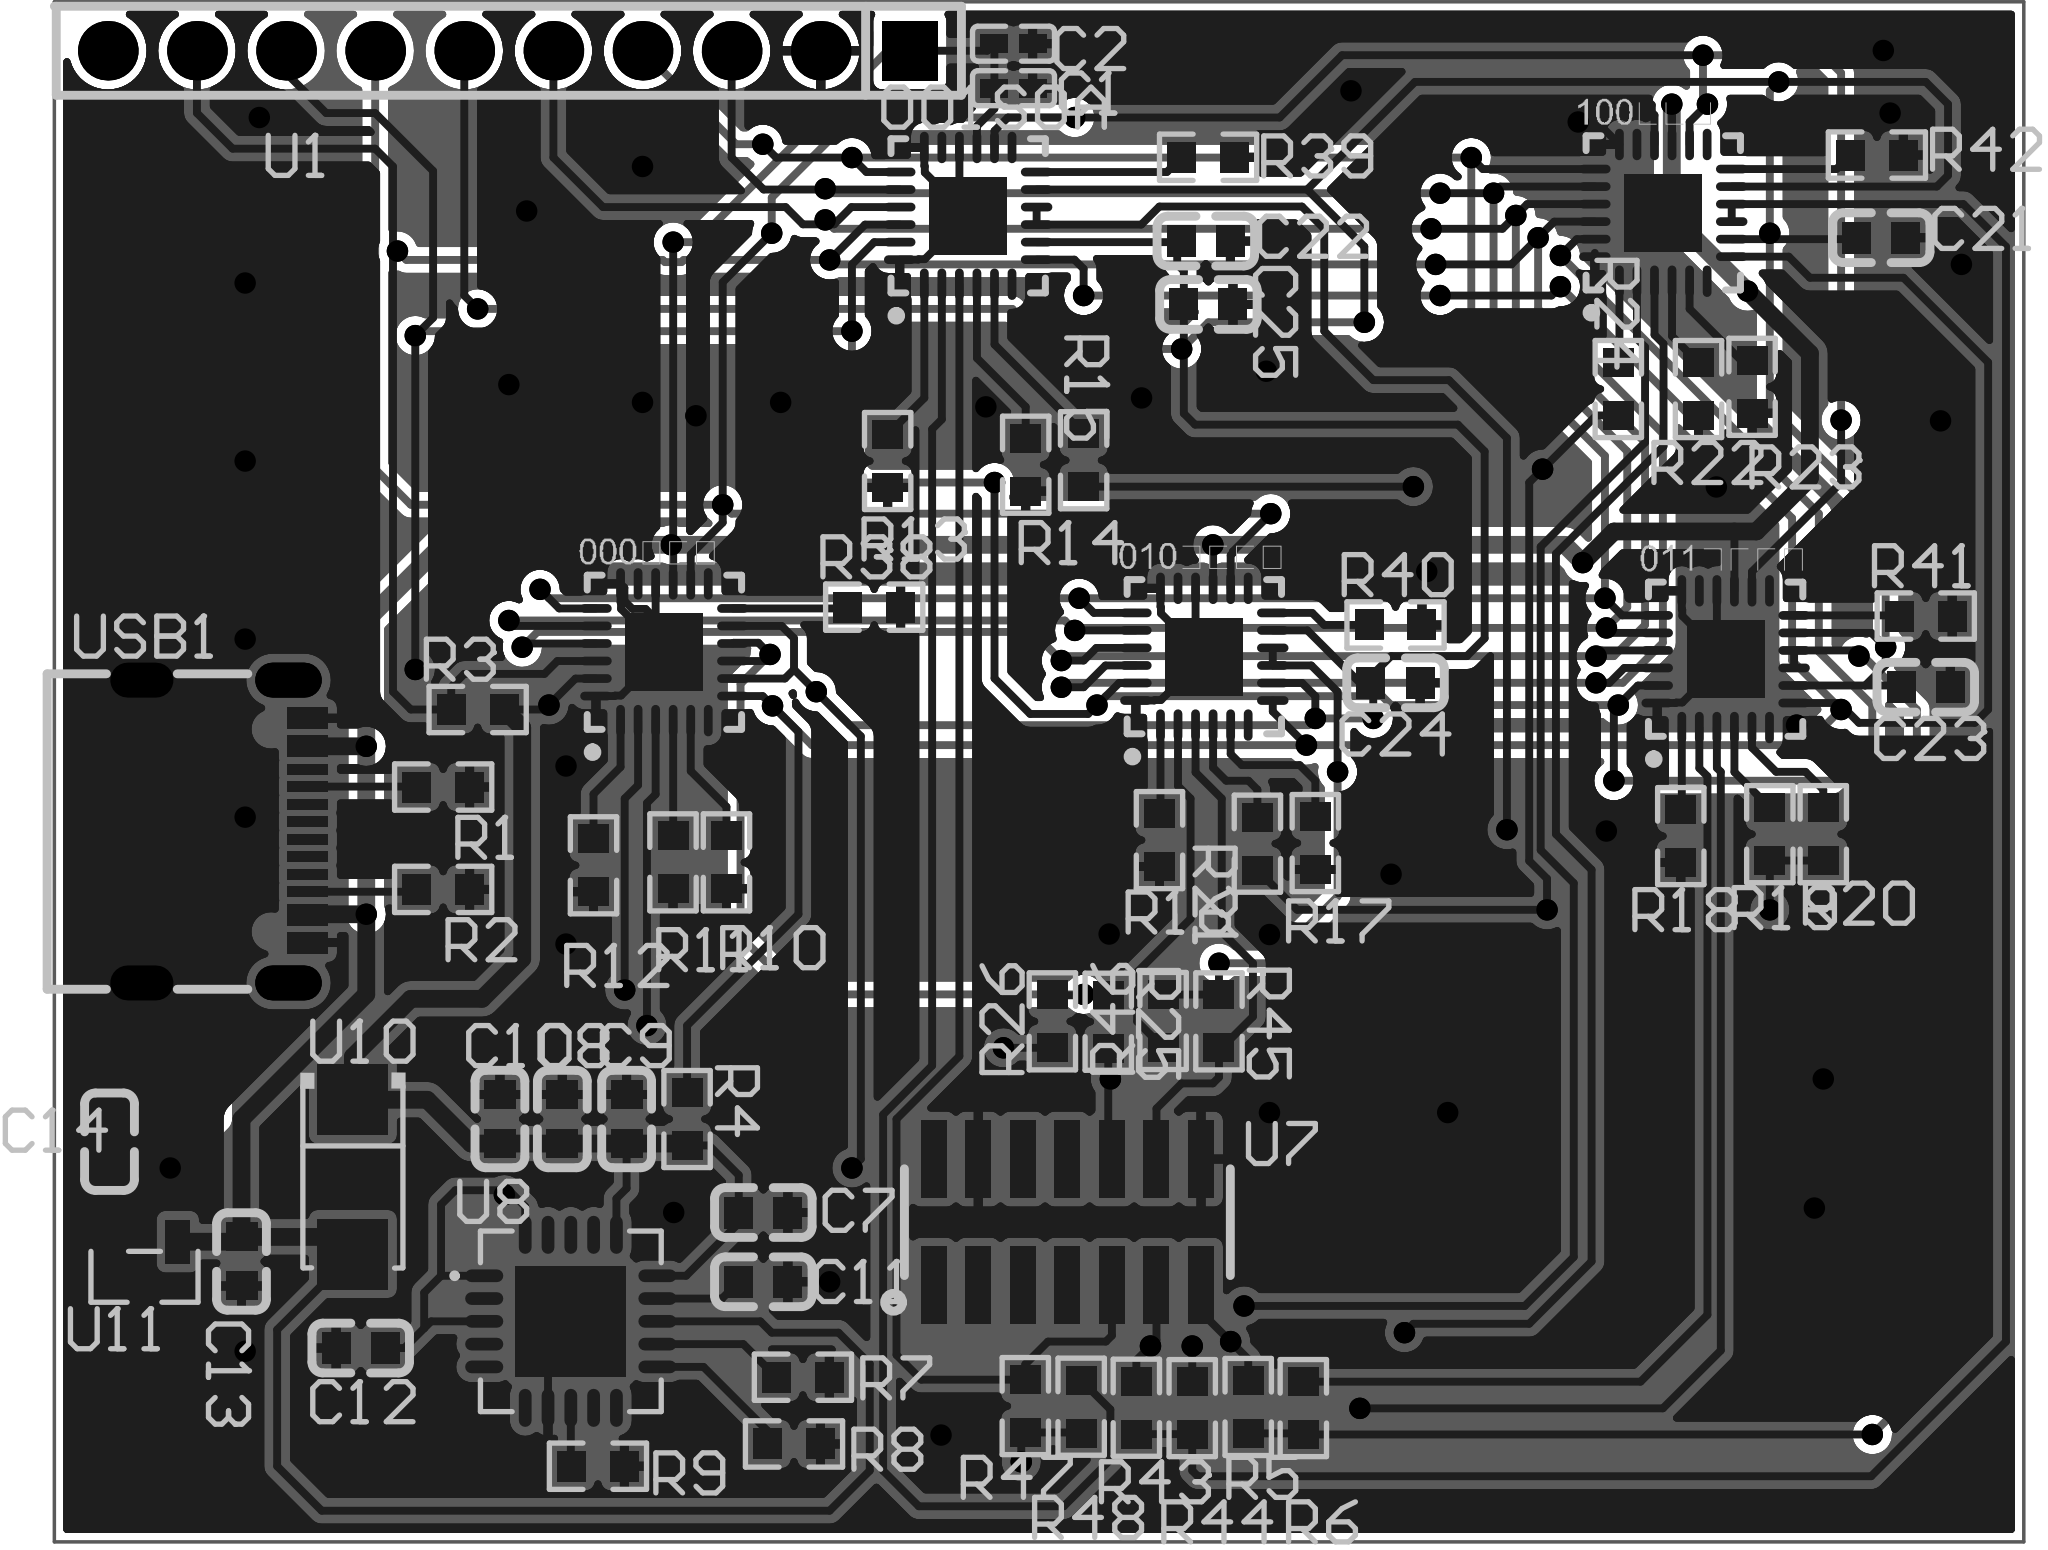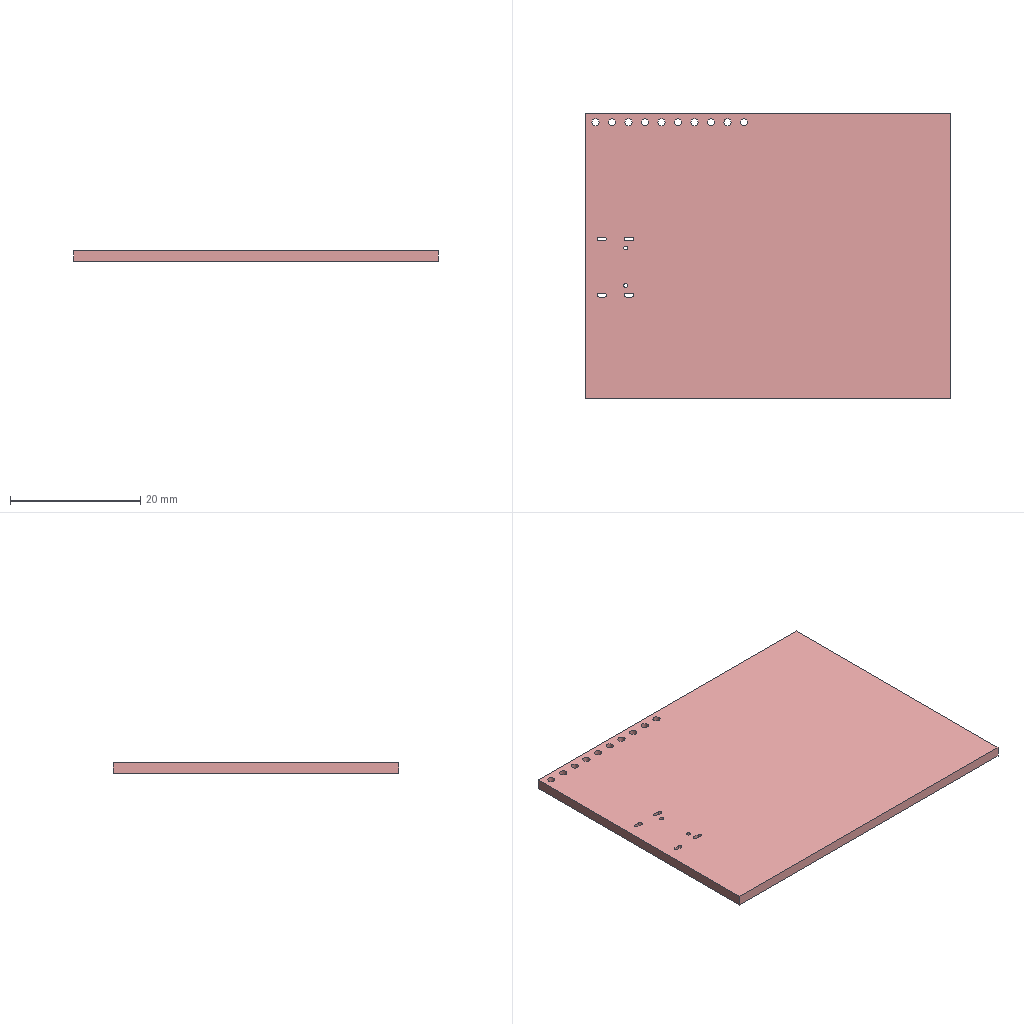Circuit board layout | Altium Designer | box 56.1 x 43.9 x 1.6 mm
Layer stack:
# Altium Designer layer stack of  (unit mm; dielectric type: 0 none, 1 core, 2 prepreg, 3 surface material)
index,name,kind,layer,copper_thickness_mm,dielectric_type,dielectric_thickness_mm,dielectric_material,dielectric_constant
0,Top Paste Mask Layer,other,,,,,,
1,Top Silkscreen Layer,other,,,,,,
2,Top Solder Mask Layer,dielectric,,,3,0.01,,3.3
3,Top Layer,copper,Top Layer,0.035,,,,
4,Dielectric1,dielectric,,,3,1.51,FR4,4.5
5,Bottom Layer,copper,Bottom Layer,0.035,,,,
6,Bottom Solder Mask Layer,dielectric,,,3,0.01,,3.3
7,Bottom Silkscreen Layer,other,,,,,,
8,Bottom Paste Mask Layer,other,,,,,,
# drill layer pairs: low layer,high layer
drill_pair,Top Layer,Bottom Layer
Part placement:
Designator,Comment,Layer,Footprint,Center-X(mm),Center-Y(mm),Rotation
000增益节,ADN8810ACPZ,TopLayer,LFCSP-24_L4.0-W4.0-P0.50-BL-EP2.3,100.7,107.171,0
001SOA,ADN8810ACPZ,TopLayer,LFCSP-24_L4.0-W4.0-P0.50-BL-EP2.3,109.358,119.623,0
010左光栅节,ADN8810ACPZ,TopLayer,LFCSP-24_L4.0-W4.0-P0.50-BL-EP2.3,116.089,107.044,0
011右光栅节,ADN8810ACPZ,TopLayer,LFCSP-24_L4.0-W4.0-P0.50-BL-EP2.3,130.948,106.973,0
100相位节,ADN8810ACPZ,TopLayer,LFCSP-24_L4.0-W4.0-P0.50-BL-EP2.3,129.17,119.708,0
C1,10uF,TopLayer,C0402,110.65,123.265,180
C2,100nF,TopLayer,C0402,110.65,124.535,180
C7,10uF,TopLayer,C0603,103.52,91.186,0
C8,10uF,TopLayer,C0603,97.79,93.853,90
C9,0.1uF,TopLayer,C0603,99.623,93.853,270
C10,0.1uF,TopLayer,C0603,96.012,93.853,270
C11,1uF,TopLayer,C0603,103.52,89.21,180
C12,10uF,TopLayer,C0603,92.043,87.319,0
C13,2.2uF,TopLayer,C0603,88.646,89.789,270
C14,2.2uF,TopLayer,C0603,84.884,93.206,270
C21,100nF,TopLayer,C0603,135.382,118.999,0
C22,100nF,TopLayer,C0603,116.132,118.903,0
C23,100nF,TopLayer,C0603,136.652,106.172,0
C24,100nF,TopLayer,C0603,121.539,106.299,0
C25,100nF,TopLayer,C0603,116.205,117.094,0
R1,5.1K,TopLayer,R0603,94.394,103.326,180
R2,5.1K,TopLayer,R0603,94.394,100.405,180
R5,3,TopLayer,R0603,117.34,85.637,90
R6,3,TopLayer,R0603,118.911,85.606,270
R7,0,TopLayer,R0603,104.648,86.487,0
R8,0,TopLayer,R0603,104.394,84.582,0
R9,0,TopLayer,R0603,98.806,83.947,0
R10,10K,TopLayer,R0603,102.469,101.176,90
R11,10K,TopLayer,R0603,100.945,101.176,90
R12,10K,TopLayer,R0603,98.679,101.092,90
R13,10K,TopLayer,R0603,107.063,112.627,90
R14,10K,TopLayer,R0603,110.998,112.522,90
R15,10K,TopLayer,R0603,112.649,112.649,90
R16,10K,TopLayer,R0603,114.81,101.811,90
R17,10K,TopLayer,R0603,119.253,101.727,90
R18,10K,TopLayer,R0603,129.669,101.925,90
R19,10K,TopLayer,R0603,132.207,101.981,90
R20,10K,TopLayer,R0603,133.731,101.981,90
R21,10K,TopLayer,R0603,117.602,101.71,90
R22,10K,TopLayer,R0603,130.175,114.681,90
R23,10K,TopLayer,R0603,131.701,114.744,90
R24,10K,TopLayer,R0603,127.889,114.681,90
R25,1.37,TopLayer,R0603,113.351,96.629,270
R26,1.37,TopLayer,R0603,111.758,96.64,90
R38,10K,TopLayer,R0603,106.68,108.458,0
R39,10K,TopLayer,R0603,116.196,121.294,0
R40,10K,TopLayer,R0603,121.539,107.95,0
R41,10K,TopLayer,R0603,136.652,108.204,0
R42,10K,TopLayer,R0603,135.26,121.358,0
R43,3,TopLayer,R0603,114.152,85.616,90
R44,3,TopLayer,R0603,115.744,85.605,270
R45,3,TopLayer,R0603,116.506,96.639,270
R46,3,TopLayer,R0603,114.914,96.65,90
R47,1.37,TopLayer,R0603,110.986,85.663,90
R48,1.37,TopLayer,R0603,112.579,85.646,270
U7,ATLS7503,TopLayer,HDR-SMD_14P-P1.27-V-F-R2-C7-LS4.8,112.185,90.91,0
U8,TPS7A4701RGWR,TopLayer,VQFN-20_L5.0-W5.0-P0.65-TL-EP,98.033,88.081,0
U10,SS310 Schottky diode SMA,TopLayer,SMA_L4.3-W2.6-LS5.1-R-RD,91.821,92.202,270
U11,REF2940AIDBZT,TopLayer,SOT-23-3_L2.9-W1.3-P1.90-LS2.4-BR,85.881,89.352,90
USB1,Type-C-16P,TopLayer,USB-C-SMD_GT-USB-7010E,88.171,102.056,270
U1,2.54mm pitch red header 1x10pin,TopLayer,HDR-TH_10P-P2.54-V-F-2,96.266,124.333,180
R3,10K,TopLayer,R0603,95.377,105.537,0
R4,10K,TopLayer,R0603,101.346,93.853,270
Pad and via stacks:
# Altium Designer via and pad stacks of  (unit mm). Each distinct definition once, with the count of objects using it.
# via: kind,start_layer,end_layer,hole_mm,diameter_mm,mode(0 simple;1 top-mid-bottom;2 full stack),diameter_per_layer,count,example_net
# pad: kind,layer,hole_mm,hole_type(0 round;1 square;2 slot),plating,top_size,top_shape(1 round;2 rect;3 octagon;9 rounded rect),mid_size,bottom_size,mode,footprint,size_per_layer,count,example
pad,Top Layer,0,0,plated,0.9x0.25,1,0.9x0.25,0.9x0.25,0,LFCSP-24_L4.0-W4.0-P0.50-BL-EP2.3,,60,000\u589E\u76CA\u8282.24
pad,Top Layer,0,0,plated,0.25x0.9,1,0.25x0.9,0.25x0.9,0,LFCSP-24_L4.0-W4.0-P0.50-BL-EP2.3,,60,000\u589E\u76CA\u8282.18
pad,Top Layer,0,0,plated,2.2x2.2,2,2.2x2.2,2.2x2.2,0,LFCSP-24_L4.0-W4.0-P0.50-BL-EP2.3,,5,000\u589E\u76CA\u8282.25
pad,Top Layer,0,0,plated,0.7901x0.54,2,0.7901x0.54,0.7901x0.54,0,C0402,,4,C1.2
pad,Top Layer,0,0,plated,0.8x0.9,2,0.8x0.9,0.8x0.9,0,C0603,,26,C7.2
pad,Top Layer,0,0,plated,0.8065x0.864,2,0.8065x0.864,0.8065x0.864,0,R0603,,74,R1.2
pad,Top Layer,0,0,plated,2.2x0.74,2,2.2x0.74,2.2x0.74,0,HDR-SMD_14P-P1.27-V-F-R2-C7-LS4.8,,14,U7.1
pad,Top Layer,0,0,plated,1.087x0.364,1,1.087x0.364,1.087x0.364,0,VQFN-20_L5.0-W5.0-P0.65-TL-EP,,10,U8.1
pad,Top Layer,0,0,plated,0.364x1.087,1,0.364x1.087,0.364x1.087,0,VQFN-20_L5.0-W5.0-P0.65-TL-EP,,10,U8.6
pad,Top Layer,0,0,plated,3.15x3.15,2,3.15x3.15,3.15x3.15,0,VQFN-20_L5.0-W5.0-P0.65-TL-EP,,1,U8.21
pad,Top Layer,0,0,plated,2x2,2,2x2,2x2,0,SMA_L4.3-W2.6-LS5.1-R-RD,,2,U10.1
pad,Top Layer,0,0,plated,1.25x0.7,2,1.25x0.7,1.25x0.7,0,SOT-23-3_L2.9-W1.3-P1.90-LS2.4-BR,,3,U11.1
pad,Top Layer,0,0,plated,0.6x1.15,2,0.6x1.15,0.6x1.15,0,USB-C-SMD_GT-USB-7010E,,4,USB1.B1A12
pad,Top Layer,0,0,plated,0.3x1.15,2,0.3x1.15,0.3x1.15,0,USB-C-SMD_GT-USB-7010E,,8,USB1.B5
pad,Multi-Layer,0.6,2,plated,1x1.9,1,1x1.9,1x1.9,0,USB-C-SMD_GT-USB-7010E,,2,USB1.1
pad,Multi-Layer,0.6,2,plated,1x1.8,1,1x1.8,1x1.8,0,USB-C-SMD_GT-USB-7010E,,2,USB1.4
pad,Multi-Layer,1.1,0,plated,1.7x1.7,1,1.7x1.7,1.7x1.7,0,HDR-TH_10P-P2.54-V-F-2,,9,U1.10
pad,Multi-Layer,1.1,0,plated,1.575x1.7,2,1.575x1.7,1.575x1.7,0,HDR-TH_10P-P2.54-V-F-2,,1,U1.1
via,Top Layer,Bottom Layer,0.3048,0.61,0,,127,3V3_OUT
Copper pours:
name,layer,net,type(0 solid;1 hatched;2 none)
Top Layer-GND,Top Layer,GND,0
Top Layer-GND 1,Top Layer,GND,0
Top Layer-GND 2,Top Layer,GND,0
Bottom Layer-GND,Bottom Layer,GND,0
Bottom Layer-GND 1,Bottom Layer,GND,0
Bottom Layer-GND 2,Bottom Layer,GND,0
Design rules, without the lines most boards share:
# Altium Designer design rules of  (exported by Altium Designer, unit mm)
# columns: name | kind | enabled | priority | scope1 | scope2 | descriptor | typed fields (field=value)
Copper_copperRegion_copperThickness1oz | 0 | disabled | 4 | All | All | Clearance Constraint (Gap=5.984mil) (Disabled)(All),(All) | gap=0.152
Copper_copperRegion_copperThickness1oz_1 | 63 | disabled | 4 | All | All | Board Clearance Constraint (Gap=0mil) (Disabled)(All) |
Copper_copperRegion_Copper_copperRegion | 0 | disabled | 5 | All | All | Clearance Constraint (Gap=5.984mil) (Disabled)(All),(All) | gap=0.152
Copper_copperRegion_Copper_copperRegion_1 | 63 | disabled | 5 | All | All | Board Clearance Constraint (Gap=0mil) (Disabled)(All) |
copperThickness1oz | 0 | enabled | 6 | All | All | Clearance Constraint (Gap=5.984mil) (All),(All) | gap=0.152
copperThickness1oz_1 | 63 | enabled | 6 | All | All | Board Clearance Constraint (Gap=0mil) (All) |
copperRegion_copperThickness1oz | 20 | disabled | 1 | All | All | Polygon Connect Rule(Relief Connect )(Conductor Width=10mil) (Relief Angle=90 Angle) (Entries=4) (Air Gap Width=10mil) (Disabled)(All),(All) | connect_style(0=relief,1=direct,2=none)=0 relief_conductor_width=0.254 relief_entries=4
copperRegion_Copper_copperRegion | 20 | disabled | 2 | All | All | Polygon Connect Rule(Relief Connect )(Conductor Width=10mil) (Relief Angle=90 Angle) (Entries=4) (Air Gap Width=10mil) (Disabled)(All),(All) | connect_style(0=relief,1=direct,2=none)=0 relief_conductor_width=0.254 relief_entries=4
copperRegion | 20 | enabled | 3 | All | All | Polygon Connect Rule(Relief Connect )(Conductor Width=10mil) (Relief Angle=90 Angle) (Entries=4) (Air Gap Width=10mil) (All),(All) | connect_style(0=relief,1=direct,2=none)=0 relief_conductor_width=0.254 relief_entries=4